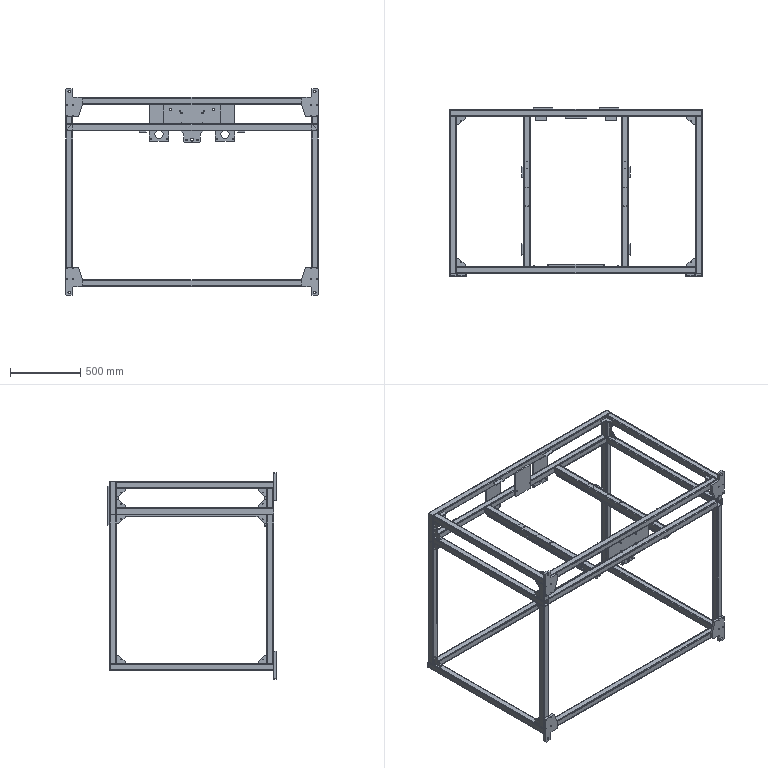Part | SolidWorks | features BaseBody 59 | 59 solids | 1094 faces | box 1800 x 1198 x 1470 mm | volume 18409114 mm3 | plane 548 | cylinder 542 | cone 4 | commonest cylinder face diameters 6.8 x192 6 x118 12 x88 5 x80 10.2 x26 8.5 x20